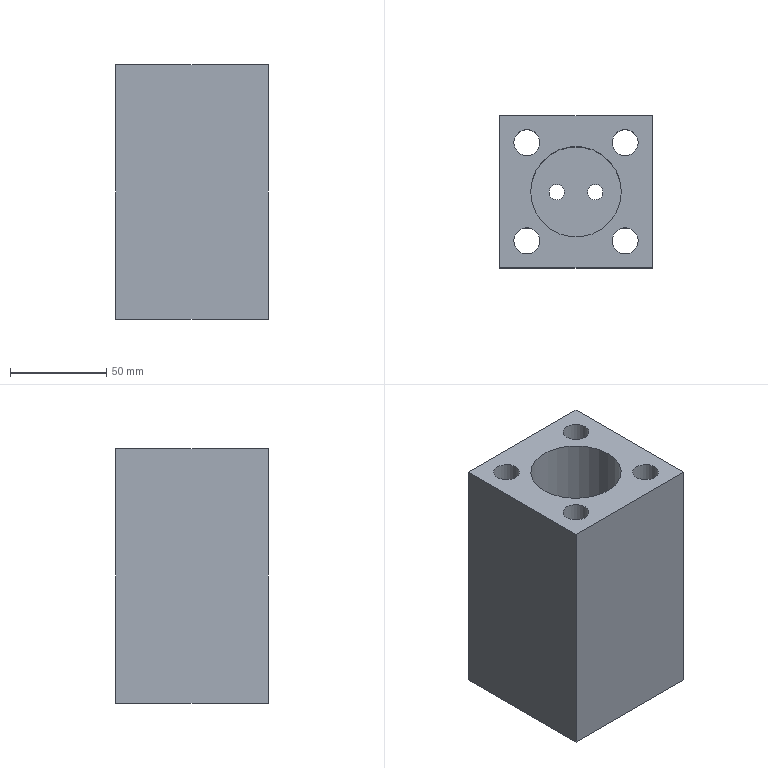Part | STEP file | lll_id4418_x_t | 1 solid | 26 faces | box 79 x 79 x 132 mm | volume 483793 mm3 | plane 13 | cylinder 13 | commonest cylinder face diameters 13.509 x4 20.007 x4 8 x2 13 x2 47 x1
STEP:
#1=CARTESIAN_POINT('',(3155.503,-196.5,-312.));
#2=VERTEX_POINT('',#1);
#3=CARTESIAN_POINT('',(3145.5,-196.5,-312.));
#4=DIRECTION('',(0.,0.,1.));
#5=DIRECTION('',(1.,0.,0.));
#6=AXIS2_PLACEMENT_3D('',#3,#4,#5);
#7=CIRCLE('',#6,10.004);
#8=EDGE_CURVE('',#2,#2,#7,.T.);
#9=ORIENTED_EDGE('',*,*,#8,.T.);
#10=EDGE_LOOP('',(#9));
#11=FACE_BOUND('',#10,.T.);
#12=CARTESIAN_POINT('',(3104.503,-196.5,-312.));
#13=VERTEX_POINT('',#12);
#14=CARTESIAN_POINT('',(3094.5,-196.5,-312.));
#15=DIRECTION('',(0.,0.,1.));
#16=DIRECTION('',(1.,0.,0.));
#17=AXIS2_PLACEMENT_3D('',#14,#15,#16);
#18=CIRCLE('',#17,10.004);
#19=EDGE_CURVE('',#13,#13,#18,.T.);
#20=ORIENTED_EDGE('',*,*,#19,.T.);
#21=EDGE_LOOP('',(#20));
#22=FACE_BOUND('',#21,.T.);
#23=CARTESIAN_POINT('',(3159.5,-210.5,-312.));
#24=VERTEX_POINT('',#23);
#25=CARTESIAN_POINT('',(3159.5,-131.5,-312.));
#26=VERTEX_POINT('',#25);
#27=CARTESIAN_POINT('',(3159.5,-171.,-312.));
#28=DIRECTION('',(0.,1.,0.));
#29=VECTOR('',#28,1.);
#30=LINE('',#27,#29);
#31=EDGE_CURVE('',#24,#26,#30,.T.);
#32=ORIENTED_EDGE('',*,*,#31,.F.);
#33=CARTESIAN_POINT('',(3080.5,-210.5,-312.));
#34=VERTEX_POINT('',#33);
#35=CARTESIAN_POINT('',(3120.,-210.5,-312.));
#36=DIRECTION('',(1.,0.,0.));
#37=VECTOR('',#36,1.);
#38=LINE('',#35,#37);
#39=EDGE_CURVE('',#34,#24,#38,.T.);
#40=ORIENTED_EDGE('',*,*,#39,.F.);
#41=CARTESIAN_POINT('',(3080.5,-131.5,-312.));
#42=VERTEX_POINT('',#41);
#43=CARTESIAN_POINT('',(3080.5,-171.,-312.));
#44=DIRECTION('',(0.,-1.,0.));
#45=VECTOR('',#44,1.);
#46=LINE('',#43,#45);
#47=EDGE_CURVE('',#42,#34,#46,.T.);
#48=ORIENTED_EDGE('',*,*,#47,.F.);
#49=CARTESIAN_POINT('',(3120.,-131.5,-312.));
#50=DIRECTION('',(-1.,0.,0.));
#51=VECTOR('',#50,1.);
#52=LINE('',#49,#51);
#53=EDGE_CURVE('',#26,#42,#52,.T.);
#54=ORIENTED_EDGE('',*,*,#53,.F.);
#55=EDGE_LOOP('',(#32,#40,#48,#54));
#56=FACE_BOUND('',#55,.T.);
#57=CARTESIAN_POINT('',(3155.503,-145.5,-312.));
#58=VERTEX_POINT('',#57);
#59=CARTESIAN_POINT('',(3145.5,-145.5,-312.));
#60=DIRECTION('',(0.,0.,1.));
#61=DIRECTION('',(1.,0.,0.));
#62=AXIS2_PLACEMENT_3D('',#59,#60,#61);
#63=CIRCLE('',#62,10.004);
#64=EDGE_CURVE('',#58,#58,#63,.T.);
#65=ORIENTED_EDGE('',*,*,#64,.T.);
#66=EDGE_LOOP('',(#65));
#67=FACE_BOUND('',#66,.T.);
#68=CARTESIAN_POINT('',(3104.503,-145.5,-312.));
#69=VERTEX_POINT('',#68);
#70=CARTESIAN_POINT('',(3094.5,-145.5,-312.));
#71=DIRECTION('',(0.,0.,1.));
#72=DIRECTION('',(1.,0.,0.));
#73=AXIS2_PLACEMENT_3D('',#70,#71,#72);
#74=CIRCLE('',#73,10.004);
#75=EDGE_CURVE('',#69,#69,#74,.T.);
#76=ORIENTED_EDGE('',*,*,#75,.T.);
#77=EDGE_LOOP('',(#76));
#78=FACE_BOUND('',#77,.T.);
#79=CARTESIAN_POINT('',(3103.5,-171.,-312.));
#80=VERTEX_POINT('',#79);
#81=CARTESIAN_POINT('',(3110.,-171.,-312.));
#82=DIRECTION('',(0.,0.,-1.));
#83=DIRECTION('',(-1.,0.,0.));
#84=AXIS2_PLACEMENT_3D('',#81,#82,#83);
#85=CIRCLE('',#84,6.5);
#86=EDGE_CURVE('',#80,#80,#85,.T.);
#87=ORIENTED_EDGE('',*,*,#86,.F.);
#88=EDGE_LOOP('',(#87));
#89=FACE_BOUND('',#88,.T.);
#90=CARTESIAN_POINT('',(3123.5,-171.,-312.));
#91=VERTEX_POINT('',#90);
#92=CARTESIAN_POINT('',(3130.,-171.,-312.));
#93=DIRECTION('',(0.,0.,1.));
#94=DIRECTION('',(-1.,0.,0.));
#95=AXIS2_PLACEMENT_3D('',#92,#93,#94);
#96=CIRCLE('',#95,6.5);
#97=EDGE_CURVE('',#91,#91,#96,.T.);
#98=ORIENTED_EDGE('',*,*,#97,.T.);
#99=EDGE_LOOP('',(#98));
#100=FACE_BOUND('',#99,.T.);
#101=CARTESIAN_POINT('',(3120.,-171.,-312.));
#102=DIRECTION('',(0.,0.,-1.));
#103=DIRECTION('',(-1.,0.,0.));
#104=AXIS2_PLACEMENT_3D('',#101,#102,#103);
#105=PLANE('',#104);
#106=ADVANCED_FACE('',(#11,#22,#56,#67,#78,#89,#100),#105,.T.);
#107=CARTESIAN_POINT('',(3126.,-171.,-292.));
#108=VERTEX_POINT('',#107);
#109=CARTESIAN_POINT('',(3130.,-171.,-292.));
#110=DIRECTION('',(0.,0.,-1.));
#111=DIRECTION('',(-1.,0.,0.));
#112=AXIS2_PLACEMENT_3D('',#109,#110,#111);
#113=CIRCLE('',#112,4.);
#114=EDGE_CURVE('',#108,#108,#113,.T.);
#115=ORIENTED_EDGE('',*,*,#114,.F.);
#116=EDGE_LOOP('',(#115));
#117=FACE_BOUND('',#116,.T.);
#118=CARTESIAN_POINT('',(3126.,-171.,-302.));
#119=VERTEX_POINT('',#118);
#120=CARTESIAN_POINT('',(3130.,-171.,-302.));
#121=DIRECTION('',(0.,0.,-1.));
#122=DIRECTION('',(-1.,0.,0.));
#123=AXIS2_PLACEMENT_3D('',#120,#121,#122);
#124=CIRCLE('',#123,4.);
#125=EDGE_CURVE('',#119,#119,#124,.T.);
#126=ORIENTED_EDGE('',*,*,#125,.T.);
#127=EDGE_LOOP('',(#126));
#128=FACE_BOUND('',#127,.T.);
#129=CARTESIAN_POINT('',(3130.,-171.,-404.));
#130=DIRECTION('',(0.,0.,1.));
#131=DIRECTION('',(1.,0.,0.));
#132=AXIS2_PLACEMENT_3D('',#129,#130,#131);
#133=CYLINDRICAL_SURFACE('',#132,4.);
#134=ADVANCED_FACE('',(#117,#128),#133,.F.);
#135=ORIENTED_EDGE('',*,*,#114,.T.);
#136=EDGE_LOOP('',(#135));
#137=FACE_BOUND('',#136,.T.);
#138=CARTESIAN_POINT('',(3096.5,-171.,-292.));
#139=VERTEX_POINT('',#138);
#140=CARTESIAN_POINT('',(3120.,-171.,-292.));
#141=DIRECTION('',(0.,0.,1.));
#142=DIRECTION('',(-1.,0.,0.));
#143=AXIS2_PLACEMENT_3D('',#140,#141,#142);
#144=CIRCLE('',#143,23.5);
#145=EDGE_CURVE('',#139,#139,#144,.T.);
#146=ORIENTED_EDGE('',*,*,#145,.T.);
#147=EDGE_LOOP('',(#146));
#148=FACE_BOUND('',#147,.T.);
#149=CARTESIAN_POINT('',(3106.,-171.,-292.));
#150=VERTEX_POINT('',#149);
#151=CARTESIAN_POINT('',(3110.,-171.,-292.));
#152=DIRECTION('',(0.,0.,1.));
#153=DIRECTION('',(-1.,0.,0.));
#154=AXIS2_PLACEMENT_3D('',#151,#152,#153);
#155=CIRCLE('',#154,4.);
#156=EDGE_CURVE('',#150,#150,#155,.T.);
#157=ORIENTED_EDGE('',*,*,#156,.F.);
#158=EDGE_LOOP('',(#157));
#159=FACE_BOUND('',#158,.T.);
#160=CARTESIAN_POINT('',(3130.8,-171.,-292.));
#161=DIRECTION('',(0.,0.,-1.));
#162=DIRECTION('',(1.,0.,0.));
#163=AXIS2_PLACEMENT_3D('',#160,#161,#162);
#164=PLANE('',#163);
#165=ADVANCED_FACE('',(#137,#148,#159),#164,.F.);
#166=CARTESIAN_POINT('',(3087.745,-145.5,-180.));
#167=VERTEX_POINT('',#166);
#168=CARTESIAN_POINT('',(3094.5,-145.5,-180.));
#169=DIRECTION('',(0.,0.,1.));
#170=DIRECTION('',(-1.,0.,0.));
#171=AXIS2_PLACEMENT_3D('',#168,#169,#170);
#172=CIRCLE('',#171,6.755);
#173=EDGE_CURVE('',#167,#167,#172,.T.);
#174=ORIENTED_EDGE('',*,*,#173,.F.);
#175=EDGE_LOOP('',(#174));
#176=FACE_BOUND('',#175,.T.);
#177=CARTESIAN_POINT('',(3138.745,-196.5,-180.));
#178=VERTEX_POINT('',#177);
#179=CARTESIAN_POINT('',(3145.5,-196.5,-180.));
#180=DIRECTION('',(0.,0.,1.));
#181=DIRECTION('',(-1.,0.,0.));
#182=AXIS2_PLACEMENT_3D('',#179,#180,#181);
#183=CIRCLE('',#182,6.755);
#184=EDGE_CURVE('',#178,#178,#183,.T.);
#185=ORIENTED_EDGE('',*,*,#184,.F.);
#186=EDGE_LOOP('',(#185));
#187=FACE_BOUND('',#186,.T.);
#188=CARTESIAN_POINT('',(3138.745,-145.5,-180.));
#189=VERTEX_POINT('',#188);
#190=CARTESIAN_POINT('',(3145.5,-145.5,-180.));
#191=DIRECTION('',(0.,0.,1.));
#192=DIRECTION('',(-1.,0.,0.));
#193=AXIS2_PLACEMENT_3D('',#190,#191,#192);
#194=CIRCLE('',#193,6.755);
#195=EDGE_CURVE('',#189,#189,#194,.T.);
#196=ORIENTED_EDGE('',*,*,#195,.F.);
#197=EDGE_LOOP('',(#196));
#198=FACE_BOUND('',#197,.T.);
#199=CARTESIAN_POINT('',(3087.745,-196.5,-180.));
#200=VERTEX_POINT('',#199);
#201=CARTESIAN_POINT('',(3094.5,-196.5,-180.));
#202=DIRECTION('',(0.,0.,1.));
#203=DIRECTION('',(-1.,0.,0.));
#204=AXIS2_PLACEMENT_3D('',#201,#202,#203);
#205=CIRCLE('',#204,6.755);
#206=EDGE_CURVE('',#200,#200,#205,.T.);
#207=ORIENTED_EDGE('',*,*,#206,.F.);
#208=EDGE_LOOP('',(#207));
#209=FACE_BOUND('',#208,.T.);
#210=CARTESIAN_POINT('',(3096.5,-171.,-180.));
#211=VERTEX_POINT('',#210);
#212=CARTESIAN_POINT('',(3120.,-171.,-180.));
#213=DIRECTION('',(0.,0.,1.));
#214=DIRECTION('',(-1.,0.,0.));
#215=AXIS2_PLACEMENT_3D('',#212,#213,#214);
#216=CIRCLE('',#215,23.5);
#217=EDGE_CURVE('',#211,#211,#216,.T.);
#218=ORIENTED_EDGE('',*,*,#217,.F.);
#219=EDGE_LOOP('',(#218));
#220=FACE_BOUND('',#219,.T.);
#221=CARTESIAN_POINT('',(3159.5,-210.5,-180.));
#222=VERTEX_POINT('',#221);
#223=CARTESIAN_POINT('',(3080.5,-210.5,-180.));
#224=VERTEX_POINT('',#223);
#225=CARTESIAN_POINT('',(3120.,-210.5,-180.));
#226=DIRECTION('',(-1.,0.,0.));
#227=VECTOR('',#226,1.);
#228=LINE('',#225,#227);
#229=EDGE_CURVE('',#222,#224,#228,.T.);
#230=ORIENTED_EDGE('',*,*,#229,.F.);
#231=CARTESIAN_POINT('',(3159.5,-131.5,-180.));
#232=VERTEX_POINT('',#231);
#233=CARTESIAN_POINT('',(3159.5,-171.,-180.));
#234=DIRECTION('',(0.,-1.,0.));
#235=VECTOR('',#234,1.);
#236=LINE('',#233,#235);
#237=EDGE_CURVE('',#232,#222,#236,.T.);
#238=ORIENTED_EDGE('',*,*,#237,.F.);
#239=CARTESIAN_POINT('',(3080.5,-131.5,-180.));
#240=VERTEX_POINT('',#239);
#241=CARTESIAN_POINT('',(3120.,-131.5,-180.));
#242=DIRECTION('',(1.,0.,0.));
#243=VECTOR('',#242,1.);
#244=LINE('',#241,#243);
#245=EDGE_CURVE('',#240,#232,#244,.T.);
#246=ORIENTED_EDGE('',*,*,#245,.F.);
#247=CARTESIAN_POINT('',(3080.5,-171.,-180.));
#248=DIRECTION('',(0.,1.,0.));
#249=VECTOR('',#248,1.);
#250=LINE('',#247,#249);
#251=EDGE_CURVE('',#224,#240,#250,.T.);
#252=ORIENTED_EDGE('',*,*,#251,.F.);
#253=EDGE_LOOP('',(#230,#238,#246,#252));
#254=FACE_BOUND('',#253,.T.);
#255=CARTESIAN_POINT('',(2132.435,-362.,-180.));
#256=DIRECTION('',(0.,0.,-1.));
#257=DIRECTION('',(-1.,0.,0.));
#258=AXIS2_PLACEMENT_3D('',#255,#256,#257);
#259=PLANE('',#258);
#260=ADVANCED_FACE('',(#176,#187,#198,#209,#220,#254),#259,.F.);
#261=CARTESIAN_POINT('',(3159.5,-210.5,-312.));
#262=DIRECTION('',(0.,0.,1.));
#263=VECTOR('',#262,1.);
#264=LINE('',#261,#263);
#265=EDGE_CURVE('',#24,#222,#264,.T.);
#266=ORIENTED_EDGE('',*,*,#265,.T.);
#267=ORIENTED_EDGE('',*,*,#229,.T.);
#268=CARTESIAN_POINT('',(3080.5,-210.5,-312.));
#269=DIRECTION('',(0.,0.,1.));
#270=VECTOR('',#269,1.);
#271=LINE('',#268,#270);
#272=EDGE_CURVE('',#34,#224,#271,.T.);
#273=ORIENTED_EDGE('',*,*,#272,.F.);
#274=ORIENTED_EDGE('',*,*,#39,.T.);
#275=EDGE_LOOP('',(#266,#267,#273,#274));
#276=FACE_OUTER_BOUND('',#275,.T.);
#277=CARTESIAN_POINT('',(3120.,-210.5,-312.));
#278=DIRECTION('',(0.,-1.,0.));
#279=DIRECTION('',(0.,0.,-1.));
#280=AXIS2_PLACEMENT_3D('',#277,#278,#279);
#281=PLANE('',#280);
#282=ADVANCED_FACE('',(#276),#281,.T.);
#283=ORIENTED_EDGE('',*,*,#272,.T.);
#284=ORIENTED_EDGE('',*,*,#251,.T.);
#285=CARTESIAN_POINT('',(3080.5,-131.5,-312.));
#286=DIRECTION('',(0.,0.,1.));
#287=VECTOR('',#286,1.);
#288=LINE('',#285,#287);
#289=EDGE_CURVE('',#42,#240,#288,.T.);
#290=ORIENTED_EDGE('',*,*,#289,.F.);
#291=ORIENTED_EDGE('',*,*,#47,.T.);
#292=EDGE_LOOP('',(#283,#284,#290,#291));
#293=FACE_OUTER_BOUND('',#292,.T.);
#294=CARTESIAN_POINT('',(3080.5,-171.,-312.));
#295=DIRECTION('',(-1.,0.,0.));
#296=DIRECTION('',(0.,0.,1.));
#297=AXIS2_PLACEMENT_3D('',#294,#295,#296);
#298=PLANE('',#297);
#299=ADVANCED_FACE('',(#293),#298,.T.);
#300=ORIENTED_EDGE('',*,*,#289,.T.);
#301=ORIENTED_EDGE('',*,*,#245,.T.);
#302=CARTESIAN_POINT('',(3159.5,-131.5,-312.));
#303=DIRECTION('',(0.,0.,1.));
#304=VECTOR('',#303,1.);
#305=LINE('',#302,#304);
#306=EDGE_CURVE('',#26,#232,#305,.T.);
#307=ORIENTED_EDGE('',*,*,#306,.F.);
#308=ORIENTED_EDGE('',*,*,#53,.T.);
#309=EDGE_LOOP('',(#300,#301,#307,#308));
#310=FACE_OUTER_BOUND('',#309,.T.);
#311=CARTESIAN_POINT('',(3120.,-131.5,-312.));
#312=DIRECTION('',(0.,1.,0.));
#313=DIRECTION('',(0.,0.,1.));
#314=AXIS2_PLACEMENT_3D('',#311,#312,#313);
#315=PLANE('',#314);
#316=ADVANCED_FACE('',(#310),#315,.T.);
#317=ORIENTED_EDGE('',*,*,#31,.T.);
#318=ORIENTED_EDGE('',*,*,#306,.T.);
#319=ORIENTED_EDGE('',*,*,#237,.T.);
#320=ORIENTED_EDGE('',*,*,#265,.F.);
#321=EDGE_LOOP('',(#317,#318,#319,#320));
#322=FACE_OUTER_BOUND('',#321,.T.);
#323=CARTESIAN_POINT('',(3159.5,-171.,-312.));
#324=DIRECTION('',(1.,0.,0.));
#325=DIRECTION('',(0.,0.,-1.));
#326=AXIS2_PLACEMENT_3D('',#323,#324,#325);
#327=PLANE('',#326);
#328=ADVANCED_FACE('',(#322),#327,.T.);
#329=ORIENTED_EDGE('',*,*,#145,.F.);
#330=EDGE_LOOP('',(#329));
#331=FACE_BOUND('',#330,.T.);
#332=ORIENTED_EDGE('',*,*,#217,.T.);
#333=EDGE_LOOP('',(#332));
#334=FACE_BOUND('',#333,.T.);
#335=CARTESIAN_POINT('',(3120.,-171.,-292.));
#336=DIRECTION('',(0.,0.,1.));
#337=DIRECTION('',(1.,0.,0.));
#338=AXIS2_PLACEMENT_3D('',#335,#336,#337);
#339=CYLINDRICAL_SURFACE('',#338,23.5);
#340=ADVANCED_FACE('',(#331,#334),#339,.F.);
#341=ORIENTED_EDGE('',*,*,#206,.T.);
#342=EDGE_LOOP('',(#341));
#343=FACE_BOUND('',#342,.T.);
#344=CARTESIAN_POINT('',(3101.255,-196.5,-215.));
#345=VERTEX_POINT('',#344);
#346=CARTESIAN_POINT('',(3094.5,-196.5,-215.));
#347=DIRECTION('',(0.,0.,1.));
#348=DIRECTION('',(1.,0.,0.));
#349=AXIS2_PLACEMENT_3D('',#346,#347,#348);
#350=CIRCLE('',#349,6.755);
#351=EDGE_CURVE('',#345,#345,#350,.T.);
#352=ORIENTED_EDGE('',*,*,#351,.F.);
#353=EDGE_LOOP('',(#352));
#354=FACE_BOUND('',#353,.T.);
#355=CARTESIAN_POINT('',(3094.5,-196.5,-317.));
#356=DIRECTION('',(0.,0.,1.));
#357=DIRECTION('',(1.,0.,0.));
#358=AXIS2_PLACEMENT_3D('',#355,#356,#357);
#359=CYLINDRICAL_SURFACE('',#358,6.755);
#360=ADVANCED_FACE('',(#343,#354),#359,.F.);
#361=ORIENTED_EDGE('',*,*,#351,.T.);
#362=EDGE_LOOP('',(#361));
#363=FACE_BOUND('',#362,.T.);
#364=CARTESIAN_POINT('',(3104.503,-196.5,-215.));
#365=VERTEX_POINT('',#364);
#366=CARTESIAN_POINT('',(3094.5,-196.5,-215.));
#367=DIRECTION('',(0.,0.,1.));
#368=DIRECTION('',(1.,0.,0.));
#369=AXIS2_PLACEMENT_3D('',#366,#367,#368);
#370=CIRCLE('',#369,10.004);
#371=EDGE_CURVE('',#365,#365,#370,.T.);
#372=ORIENTED_EDGE('',*,*,#371,.F.);
#373=EDGE_LOOP('',(#372));
#374=FACE_BOUND('',#373,.T.);
#375=CARTESIAN_POINT('',(3094.5,-196.5,-215.));
#376=DIRECTION('',(0.,0.,1.));
#377=DIRECTION('',(1.,0.,0.));
#378=AXIS2_PLACEMENT_3D('',#375,#376,#377);
#379=PLANE('',#378);
#380=ADVANCED_FACE('',(#363,#374),#379,.F.);
#381=ORIENTED_EDGE('',*,*,#371,.T.);
#382=EDGE_LOOP('',(#381));
#383=FACE_BOUND('',#382,.T.);
#384=ORIENTED_EDGE('',*,*,#19,.F.);
#385=EDGE_LOOP('',(#384));
#386=FACE_BOUND('',#385,.T.);
#387=CARTESIAN_POINT('',(3094.5,-196.5,-312.));
#388=DIRECTION('',(0.,0.,1.));
#389=DIRECTION('',(1.,0.,0.));
#390=AXIS2_PLACEMENT_3D('',#387,#388,#389);
#391=CYLINDRICAL_SURFACE('',#390,10.004);
#392=ADVANCED_FACE('',(#383,#386),#391,.F.);
#393=ORIENTED_EDGE('',*,*,#195,.T.);
#394=EDGE_LOOP('',(#393));
#395=FACE_BOUND('',#394,.T.);
#396=CARTESIAN_POINT('',(3152.255,-145.5,-215.));
#397=VERTEX_POINT('',#396);
#398=CARTESIAN_POINT('',(3145.5,-145.5,-215.));
#399=DIRECTION('',(0.,0.,1.));
#400=DIRECTION('',(1.,0.,0.));
#401=AXIS2_PLACEMENT_3D('',#398,#399,#400);
#402=CIRCLE('',#401,6.755);
#403=EDGE_CURVE('',#397,#397,#402,.T.);
#404=ORIENTED_EDGE('',*,*,#403,.F.);
#405=EDGE_LOOP('',(#404));
#406=FACE_BOUND('',#405,.T.);
#407=CARTESIAN_POINT('',(3145.5,-145.5,-317.));
#408=DIRECTION('',(0.,0.,1.));
#409=DIRECTION('',(1.,0.,0.));
#410=AXIS2_PLACEMENT_3D('',#407,#408,#409);
#411=CYLINDRICAL_SURFACE('',#410,6.755);
#412=ADVANCED_FACE('',(#395,#406),#411,.F.);
#413=ORIENTED_EDGE('',*,*,#403,.T.);
#414=EDGE_LOOP('',(#413));
#415=FACE_BOUND('',#414,.T.);
#416=CARTESIAN_POINT('',(3155.503,-145.5,-215.));
#417=VERTEX_POINT('',#416);
#418=CARTESIAN_POINT('',(3145.5,-145.5,-215.));
#419=DIRECTION('',(0.,0.,1.));
#420=DIRECTION('',(1.,0.,0.));
#421=AXIS2_PLACEMENT_3D('',#418,#419,#420);
#422=CIRCLE('',#421,10.004);
#423=EDGE_CURVE('',#417,#417,#422,.T.);
#424=ORIENTED_EDGE('',*,*,#423,.F.);
#425=EDGE_LOOP('',(#424));
#426=FACE_BOUND('',#425,.T.);
#427=CARTESIAN_POINT('',(3145.5,-145.5,-215.));
#428=DIRECTION('',(0.,0.,1.));
#429=DIRECTION('',(1.,0.,0.));
#430=AXIS2_PLACEMENT_3D('',#427,#428,#429);
#431=PLANE('',#430);
#432=ADVANCED_FACE('',(#415,#426),#431,.F.);
#433=ORIENTED_EDGE('',*,*,#423,.T.);
#434=EDGE_LOOP('',(#433));
#435=FACE_BOUND('',#434,.T.);
#436=ORIENTED_EDGE('',*,*,#64,.F.);
#437=EDGE_LOOP('',(#436));
#438=FACE_BOUND('',#437,.T.);
#439=CARTESIAN_POINT('',(3145.5,-145.5,-312.));
#440=DIRECTION('',(0.,0.,1.));
#441=DIRECTION('',(1.,0.,0.));
#442=AXIS2_PLACEMENT_3D('',#439,#440,#441);
#443=CYLINDRICAL_SURFACE('',#442,10.004);
#444=ADVANCED_FACE('',(#435,#438),#443,.F.);
#445=ORIENTED_EDGE('',*,*,#184,.T.);
#446=EDGE_LOOP('',(#445));
#447=FACE_BOUND('',#446,.T.);
#448=CARTESIAN_POINT('',(3152.255,-196.5,-215.));
#449=VERTEX_POINT('',#448);
#450=CARTESIAN_POINT('',(3145.5,-196.5,-215.));
#451=DIRECTION('',(0.,0.,1.));
#452=DIRECTION('',(1.,0.,0.));
#453=AXIS2_PLACEMENT_3D('',#450,#451,#452);
#454=CIRCLE('',#453,6.755);
#455=EDGE_CURVE('',#449,#449,#454,.T.);
#456=ORIENTED_EDGE('',*,*,#455,.F.);
#457=EDGE_LOOP('',(#456));
#458=FACE_BOUND('',#457,.T.);
#459=CARTESIAN_POINT('',(3145.5,-196.5,-317.));
#460=DIRECTION('',(0.,0.,1.));
#461=DIRECTION('',(1.,0.,0.));
#462=AXIS2_PLACEMENT_3D('',#459,#460,#461);
#463=CYLINDRICAL_SURFACE('',#462,6.755);
#464=ADVANCED_FACE('',(#447,#458),#463,.F.);
#465=ORIENTED_EDGE('',*,*,#455,.T.);
#466=EDGE_LOOP('',(#465));
#467=FACE_BOUND('',#466,.T.);
#468=CARTESIAN_POINT('',(3155.503,-196.5,-215.));
#469=VERTEX_POINT('',#468);
#470=CARTESIAN_POINT('',(3145.5,-196.5,-215.));
#471=DIRECTION('',(0.,0.,1.));
#472=DIRECTION('',(1.,0.,0.));
#473=AXIS2_PLACEMENT_3D('',#470,#471,#472);
#474=CIRCLE('',#473,10.004);
#475=EDGE_CURVE('',#469,#469,#474,.T.);
#476=ORIENTED_EDGE('',*,*,#475,.F.);
#477=EDGE_LOOP('',(#476));
#478=FACE_BOUND('',#477,.T.);
#479=CARTESIAN_POINT('',(3145.5,-196.5,-215.));
#480=DIRECTION('',(0.,0.,1.));
#481=DIRECTION('',(1.,0.,0.));
#482=AXIS2_PLACEMENT_3D('',#479,#480,#481);
#483=PLANE('',#482);
#484=ADVANCED_FACE('',(#467,#478),#483,.F.);
#485=ORIENTED_EDGE('',*,*,#475,.T.);
#486=EDGE_LOOP('',(#485));
#487=FACE_BOUND('',#486,.T.);
#488=ORIENTED_EDGE('',*,*,#8,.F.);
#489=EDGE_LOOP('',(#488));
#490=FACE_BOUND('',#489,.T.);
#491=CARTESIAN_POINT('',(3145.5,-196.5,-312.));
#492=DIRECTION('',(0.,0.,1.));
#493=DIRECTION('',(1.,0.,0.));
#494=AXIS2_PLACEMENT_3D('',#491,#492,#493);
#495=CYLINDRICAL_SURFACE('',#494,10.004);
#496=ADVANCED_FACE('',(#487,#490),#495,.F.);
#497=ORIENTED_EDGE('',*,*,#173,.T.);
#498=EDGE_LOOP('',(#497));
#499=FACE_BOUND('',#498,.T.);
#500=CARTESIAN_POINT('',(3101.255,-145.5,-215.));
#501=VERTEX_POINT('',#500);
#502=CARTESIAN_POINT('',(3094.5,-145.5,-215.));
#503=DIRECTION('',(0.,0.,1.));
#504=DIRECTION('',(1.,0.,0.));
#505=AXIS2_PLACEMENT_3D('',#502,#503,#504);
#506=CIRCLE('',#505,6.755);
#507=EDGE_CURVE('',#501,#501,#506,.T.);
#508=ORIENTED_EDGE('',*,*,#507,.F.);
#509=EDGE_LOOP('',(#508));
#510=FACE_BOUND('',#509,.T.);
#511=CARTESIAN_POINT('',(3094.5,-145.5,-317.));
#512=DIRECTION('',(0.,0.,1.));
#513=DIRECTION('',(1.,0.,0.));
#514=AXIS2_PLACEMENT_3D('',#511,#512,#513);
#515=CYLINDRICAL_SURFACE('',#514,6.755);
#516=ADVANCED_FACE('',(#499,#510),#515,.F.);
#517=ORIENTED_EDGE('',*,*,#507,.T.);
#518=EDGE_LOOP('',(#517));
#519=FACE_BOUND('',#518,.T.);
#520=CARTESIAN_POINT('',(3104.503,-145.5,-215.));
#521=VERTEX_POINT('',#520);
#522=CARTESIAN_POINT('',(3094.5,-145.5,-215.));
#523=DIRECTION('',(0.,0.,1.));
#524=DIRECTION('',(1.,0.,0.));
#525=AXIS2_PLACEMENT_3D('',#522,#523,#524);
#526=CIRCLE('',#525,10.004);
#527=EDGE_CURVE('',#521,#521,#526,.T.);
#528=ORIENTED_EDGE('',*,*,#527,.F.);
#529=EDGE_LOOP('',(#528));
#530=FACE_BOUND('',#529,.T.);
#531=CARTESIAN_POINT('',(3094.5,-145.5,-215.));
#532=DIRECTION('',(0.,0.,1.));
#533=DIRECTION('',(1.,0.,0.));
#534=AXIS2_PLACEMENT_3D('',#531,#532,#533);
#535=PLANE('',#534);
#536=ADVANCED_FACE('',(#519,#530),#535,.F.);
#537=ORIENTED_EDGE('',*,*,#527,.T.);
#538=EDGE_LOOP('',(#537));
#539=FACE_BOUND('',#538,.T.);
#540=ORIENTED_EDGE('',*,*,#75,.F.);
#541=EDGE_LOOP('',(#540));
#542=FACE_BOUND('',#541,.T.);
#543=CARTESIAN_POINT('',(3094.5,-145.5,-312.));
#544=DIRECTION('',(0.,0.,1.));
#545=DIRECTION('',(1.,0.,0.));
#546=AXIS2_PLACEMENT_3D('',#543,#544,#545);
#547=CYLINDRICAL_SURFACE('',#546,10.004);
#548=ADVANCED_FACE('',(#539,#542),#547,.F.);
#549=CARTESIAN_POINT('',(3114.,-171.,-302.));
#550=VERTEX_POINT('',#549);
#551=CARTESIAN_POINT('',(3110.,-171.,-302.));
#552=DIRECTION('',(0.,0.,-1.));
#553=DIRECTION('',(1.,0.,0.));
#554=AXIS2_PLACEMENT_3D('',#551,#552,#553);
#555=CIRCLE('',#554,4.);
#556=EDGE_CURVE('',#550,#550,#555,.T.);
#557=ORIENTED_EDGE('',*,*,#556,.T.);
#558=EDGE_LOOP('',(#557));
#559=FACE_BOUND('',#558,.T.);
#560=ORIENTED_EDGE('',*,*,#156,.T.);
#561=EDGE_LOOP('',(#560));
#562=FACE_BOUND('',#561,.T.);
#563=CARTESIAN_POINT('',(3110.,-171.,-404.));
#564=DIRECTION('',(0.,0.,1.));
#565=DIRECTION('',(1.,0.,0.));
#566=AXIS2_PLACEMENT_3D('',#563,#564,#565);
#567=CYLINDRICAL_SURFACE('',#566,4.);
#568=ADVANCED_FACE('',(#559,#562),#567,.F.);
#569=CARTESIAN_POINT('',(3116.5,-171.,-302.));
#570=VERTEX_POINT('',#569);
#571=CARTESIAN_POINT('',(3110.,-171.,-302.));
#572=DIRECTION('',(0.,0.,-1.));
#573=DIRECTION('',(1.,0.,0.));
#574=AXIS2_PLACEMENT_3D('',#571,#572,#573);
#575=CIRCLE('',#574,6.5);
#576=EDGE_CURVE('',#570,#570,#575,.T.);
#577=ORIENTED_EDGE('',*,*,#576,.T.);
#578=EDGE_LOOP('',(#577));
#579=FACE_BOUND('',#578,.T.);
#580=ORIENTED_EDGE('',*,*,#556,.F.);
#581=EDGE_LOOP('',(#580));
#582=FACE_BOUND('',#581,.T.);
#583=CARTESIAN_POINT('',(3110.,-171.,-302.));
#584=DIRECTION('',(0.,0.,1.));
#585=DIRECTION('',(1.,0.,0.));
#586=AXIS2_PLACEMENT_3D('',#583,#584,#585);
#587=PLANE('',#586);
#588=ADVANCED_FACE('',(#579,#582),#587,.F.);
#589=ORIENTED_EDGE('',*,*,#86,.T.);
#590=EDGE_LOOP('',(#589));
#591=FACE_BOUND('',#590,.T.);
#592=ORIENTED_EDGE('',*,*,#576,.F.);
#593=EDGE_LOOP('',(#592));
#594=FACE_BOUND('',#593,.T.);
#595=CARTESIAN_POINT('',(3110.,-171.,-404.));
#596=DIRECTION('',(0.,0.,1.));
#597=DIRECTION('',(1.,0.,0.));
#598=AXIS2_PLACEMENT_3D('',#595,#596,#597);
#599=CYLINDRICAL_SURFACE('',#598,6.5);
#600=ADVANCED_FACE('',(#591,#594),#599,.F.);
#601=ORIENTED_EDGE('',*,*,#97,.F.);
#602=EDGE_LOOP('',(#601));
#603=FACE_BOUND('',#602,.T.);
#604=CARTESIAN_POINT('',(3123.5,-171.,-302.));
#605=VERTEX_POINT('',#604);
#606=CARTESIAN_POINT('',(3130.,-171.,-302.));
#607=DIRECTION('',(0.,0.,1.));
#608=DIRECTION('',(-1.,0.,0.));
#609=AXIS2_PLACEMENT_3D('',#606,#607,#608);
#610=CIRCLE('',#609,6.5);
#611=EDGE_CURVE('',#605,#605,#610,.T.);
#612=ORIENTED_EDGE('',*,*,#611,.T.);
#613=EDGE_LOOP('',(#612));
#614=FACE_BOUND('',#613,.T.);
#615=CARTESIAN_POINT('',(3130.,-171.,-404.));
#616=DIRECTION('',(0.,0.,1.));
#617=DIRECTION('',(1.,0.,0.));
#618=AXIS2_PLACEMENT_3D('',#615,#616,#617);
#619=CYLINDRICAL_SURFACE('',#618,6.5);
#620=ADVANCED_FACE('',(#603,#614),#619,.F.);
#621=ORIENTED_EDGE('',*,*,#125,.F.);
#622=EDGE_LOOP('',(#621));
#623=FACE_BOUND('',#622,.T.);
#624=ORIENTED_EDGE('',*,*,#611,.F.);
#625=EDGE_LOOP('',(#624));
#626=FACE_BOUND('',#625,.T.);
#627=CARTESIAN_POINT('',(3130.,-171.,-302.));
#628=DIRECTION('',(0.,0.,-1.));
#629=DIRECTION('',(-1.,0.,0.));
#630=AXIS2_PLACEMENT_3D('',#627,#628,#629);
#631=PLANE('',#630);
#632=ADVANCED_FACE('',(#623,#626),#631,.T.);
#633=CLOSED_SHELL('',(#106,#134,#165,#260,#282,#299,#316,#328,#340,#360,#380,#392,#412,#432,#444,#464,#484,#496,#516,#536,#548,#568,#588,#600,#620,#632));
#634=MANIFOLD_SOLID_BREP('',#633);
#635=(LENGTH_UNIT()NAMED_UNIT(*)SI_UNIT(.MILLI.,.METRE.));
#636=UNCERTAINTY_MEASURE_WITH_UNIT(LENGTH_MEASURE(0.00002),#635,'','');
#637=(NAMED_UNIT(*)PLANE_ANGLE_UNIT()SI_UNIT($,.RADIAN.));
#638=PLANE_ANGLE_MEASURE_WITH_UNIT(PLANE_ANGLE_MEASURE(0.01745),#637);
#639=DIMENSIONAL_EXPONENTS(0.,0.,0.,0.,0.,0.,0.);
#640=(CONVERSION_BASED_UNIT('DEGREE',#638)NAMED_UNIT(#639)PLANE_ANGLE_UNIT());
#641=(NAMED_UNIT(*)SI_UNIT($,.STERADIAN.)SOLID_ANGLE_UNIT());
#642=(GEOMETRIC_REPRESENTATION_CONTEXT(3)GLOBAL_UNCERTAINTY_ASSIGNED_CONTEXT((#636))GLOBAL_UNIT_ASSIGNED_CONTEXT((#635,#640,#641))REPRESENTATION_CONTEXT('',''));
#643=ADVANCED_BREP_SHAPE_REPRESENTATION('',(#634),#642);